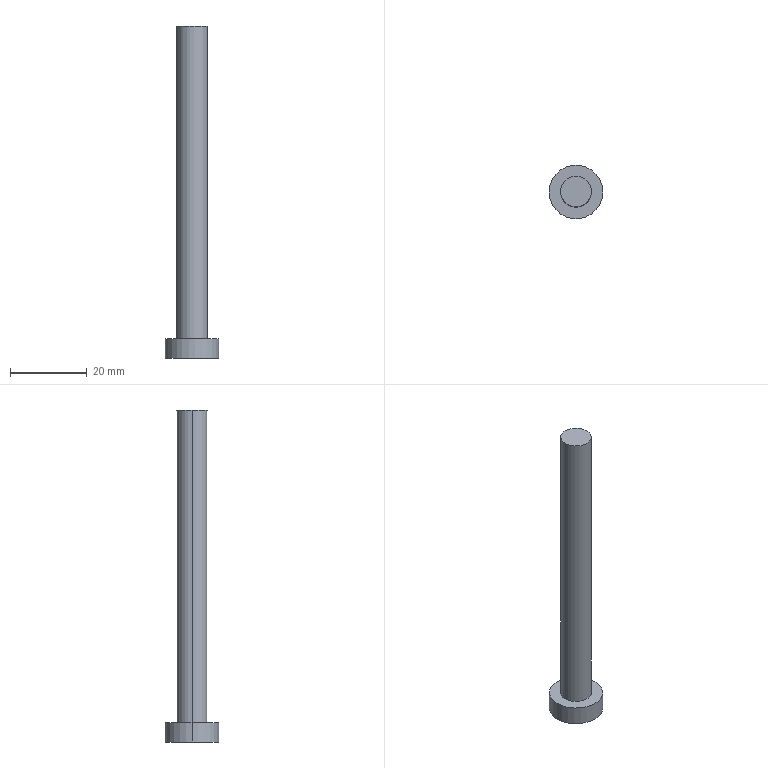Part | Creo | 1 solid | 120 faces | box 14 x 14 x 86.665 mm | volume 4873 mm3 | other 81 | plane 34 | cylinder 5 | commonest cylinder face diameters 8 x2 14 x2 30.388 x1